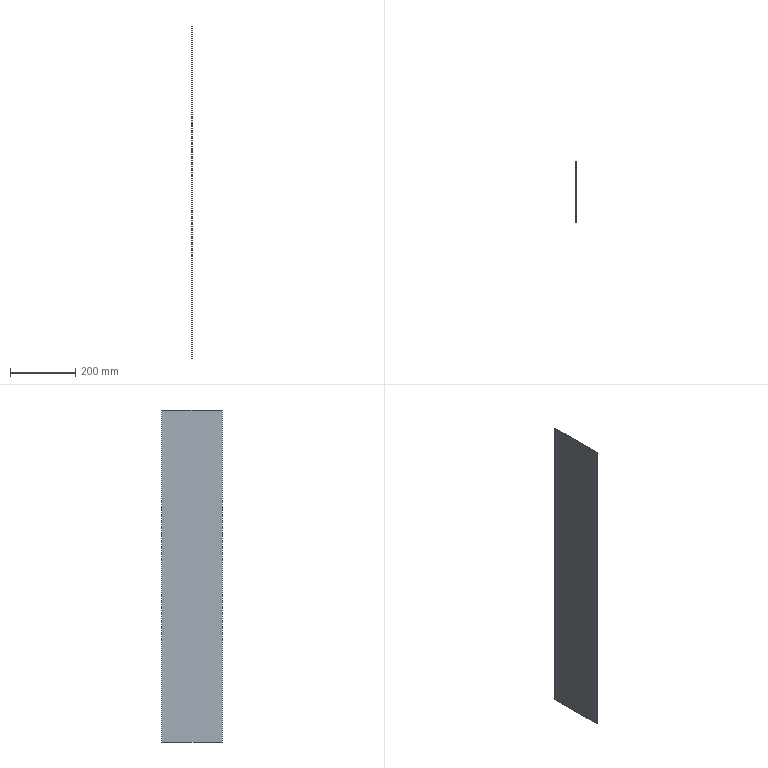Part | SolidWorks | 1 solid | 6 faces | box 1.5 x 185 x 1020 mm | volume 283050 mm3 | plane 6
STEP:
#1=CARTESIAN_POINT('',(0.,92.5,510.));
#2=VERTEX_POINT('',#1);
#3=CARTESIAN_POINT('',(0.,-92.5,510.));
#4=VERTEX_POINT('',#3);
#5=CARTESIAN_POINT('',(0.,-92.5,510.));
#6=DIRECTION('',(0.,-1.,0.));
#7=VECTOR('',#6,1000.);
#8=LINE('',#5,#7);
#9=EDGE_CURVE('',#2,#4,#8,.T.);
#10=ORIENTED_EDGE('',*,*,#9,.F.);
#11=CARTESIAN_POINT('',(-1.5,92.5,510.));
#12=VERTEX_POINT('',#11);
#13=CARTESIAN_POINT('',(-1.5,92.5,510.));
#14=DIRECTION('',(1.,0.,0.));
#15=VECTOR('',#14,1000.);
#16=LINE('',#13,#15);
#17=EDGE_CURVE('',#12,#2,#16,.T.);
#18=ORIENTED_EDGE('',*,*,#17,.F.);
#19=CARTESIAN_POINT('',(-1.5,-92.5,510.));
#20=VERTEX_POINT('',#19);
#21=CARTESIAN_POINT('',(-1.5,-92.5,510.));
#22=DIRECTION('',(0.,-1.,0.));
#23=VECTOR('',#22,1000.);
#24=LINE('',#21,#23);
#25=EDGE_CURVE('',#12,#20,#24,.T.);
#26=ORIENTED_EDGE('',*,*,#25,.T.);
#27=CARTESIAN_POINT('',(-1.5,-92.5,510.));
#28=DIRECTION('',(1.,0.,0.));
#29=VECTOR('',#28,1000.);
#30=LINE('',#27,#29);
#31=EDGE_CURVE('',#20,#4,#30,.T.);
#32=ORIENTED_EDGE('',*,*,#31,.T.);
#33=EDGE_LOOP('',(#10,#18,#26,#32));
#34=FACE_OUTER_BOUND('',#33,.T.);
#35=CARTESIAN_POINT('',(-1.5,-92.5,510.));
#36=DIRECTION('',(0.,0.,1.));
#37=DIRECTION('',(1.,0.,0.));
#38=AXIS2_PLACEMENT_3D('',#35,#36,#37);
#39=PLANE('',#38);
#40=ADVANCED_FACE('',(#34),#39,.T.);
#41=CARTESIAN_POINT('',(0.,92.5,-510.));
#42=VERTEX_POINT('',#41);
#43=CARTESIAN_POINT('',(0.,92.5,-510.));
#44=DIRECTION('',(0.,0.,1.));
#45=VECTOR('',#44,1000.);
#46=LINE('',#43,#45);
#47=EDGE_CURVE('',#42,#2,#46,.T.);
#48=ORIENTED_EDGE('',*,*,#47,.F.);
#49=CARTESIAN_POINT('',(-1.5,92.5,-510.));
#50=VERTEX_POINT('',#49);
#51=CARTESIAN_POINT('',(-1.5,92.5,-510.));
#52=DIRECTION('',(1.,0.,0.));
#53=VECTOR('',#52,1000.);
#54=LINE('',#51,#53);
#55=EDGE_CURVE('',#50,#42,#54,.T.);
#56=ORIENTED_EDGE('',*,*,#55,.F.);
#57=CARTESIAN_POINT('',(-1.5,92.5,-510.));
#58=DIRECTION('',(0.,0.,1.));
#59=VECTOR('',#58,1000.);
#60=LINE('',#57,#59);
#61=EDGE_CURVE('',#50,#12,#60,.T.);
#62=ORIENTED_EDGE('',*,*,#61,.T.);
#63=ORIENTED_EDGE('',*,*,#17,.T.);
#64=EDGE_LOOP('',(#48,#56,#62,#63));
#65=FACE_OUTER_BOUND('',#64,.T.);
#66=CARTESIAN_POINT('',(-1.5,92.5,-510.));
#67=DIRECTION('',(0.,1.,0.));
#68=DIRECTION('',(0.,0.,1.));
#69=AXIS2_PLACEMENT_3D('',#66,#67,#68);
#70=PLANE('',#69);
#71=ADVANCED_FACE('',(#65),#70,.T.);
#72=CARTESIAN_POINT('',(0.,-92.5,-510.));
#73=VERTEX_POINT('',#72);
#74=CARTESIAN_POINT('',(0.,-92.5,-510.));
#75=DIRECTION('',(0.,1.,0.));
#76=VECTOR('',#75,1000.);
#77=LINE('',#74,#76);
#78=EDGE_CURVE('',#73,#42,#77,.T.);
#79=ORIENTED_EDGE('',*,*,#78,.F.);
#80=CARTESIAN_POINT('',(-1.5,-92.5,-510.));
#81=VERTEX_POINT('',#80);
#82=CARTESIAN_POINT('',(-1.5,-92.5,-510.));
#83=DIRECTION('',(1.,0.,0.));
#84=VECTOR('',#83,1000.);
#85=LINE('',#82,#84);
#86=EDGE_CURVE('',#81,#73,#85,.T.);
#87=ORIENTED_EDGE('',*,*,#86,.F.);
#88=CARTESIAN_POINT('',(-1.5,-92.5,-510.));
#89=DIRECTION('',(0.,1.,0.));
#90=VECTOR('',#89,1000.);
#91=LINE('',#88,#90);
#92=EDGE_CURVE('',#81,#50,#91,.T.);
#93=ORIENTED_EDGE('',*,*,#92,.T.);
#94=ORIENTED_EDGE('',*,*,#55,.T.);
#95=EDGE_LOOP('',(#79,#87,#93,#94));
#96=FACE_OUTER_BOUND('',#95,.T.);
#97=CARTESIAN_POINT('',(-1.5,-92.5,-510.));
#98=DIRECTION('',(0.,0.,-1.));
#99=DIRECTION('',(-1.,0.,0.));
#100=AXIS2_PLACEMENT_3D('',#97,#98,#99);
#101=PLANE('',#100);
#102=ADVANCED_FACE('',(#96),#101,.T.);
#103=CARTESIAN_POINT('',(0.,-92.5,-510.));
#104=DIRECTION('',(0.,0.,-1.));
#105=VECTOR('',#104,1000.);
#106=LINE('',#103,#105);
#107=EDGE_CURVE('',#4,#73,#106,.T.);
#108=ORIENTED_EDGE('',*,*,#107,.F.);
#109=ORIENTED_EDGE('',*,*,#31,.F.);
#110=CARTESIAN_POINT('',(-1.5,-92.5,-510.));
#111=DIRECTION('',(0.,0.,-1.));
#112=VECTOR('',#111,1000.);
#113=LINE('',#110,#112);
#114=EDGE_CURVE('',#20,#81,#113,.T.);
#115=ORIENTED_EDGE('',*,*,#114,.T.);
#116=ORIENTED_EDGE('',*,*,#86,.T.);
#117=EDGE_LOOP('',(#108,#109,#115,#116));
#118=FACE_OUTER_BOUND('',#117,.T.);
#119=CARTESIAN_POINT('',(-1.5,-92.5,-510.));
#120=DIRECTION('',(0.,-1.,0.));
#121=DIRECTION('',(0.,0.,-1.));
#122=AXIS2_PLACEMENT_3D('',#119,#120,#121);
#123=PLANE('',#122);
#124=ADVANCED_FACE('',(#118),#123,.T.);
#125=ORIENTED_EDGE('',*,*,#25,.F.);
#126=ORIENTED_EDGE('',*,*,#61,.F.);
#127=ORIENTED_EDGE('',*,*,#92,.F.);
#128=ORIENTED_EDGE('',*,*,#114,.F.);
#129=EDGE_LOOP('',(#125,#126,#127,#128));
#130=FACE_OUTER_BOUND('',#129,.T.);
#131=CARTESIAN_POINT('',(-1.5,0.,0.));
#132=DIRECTION('',(1.,0.,0.));
#133=DIRECTION('',(0.,0.,-1.));
#134=AXIS2_PLACEMENT_3D('',#131,#132,#133);
#135=PLANE('',#134);
#136=ADVANCED_FACE('',(#130),#135,.F.);
#137=ORIENTED_EDGE('',*,*,#9,.T.);
#138=ORIENTED_EDGE('',*,*,#107,.T.);
#139=ORIENTED_EDGE('',*,*,#78,.T.);
#140=ORIENTED_EDGE('',*,*,#47,.T.);
#141=EDGE_LOOP('',(#137,#138,#139,#140));
#142=FACE_OUTER_BOUND('',#141,.T.);
#143=CARTESIAN_POINT('',(0.,0.,0.));
#144=DIRECTION('',(1.,0.,0.));
#145=DIRECTION('',(0.,0.,-1.));
#146=AXIS2_PLACEMENT_3D('',#143,#144,#145);
#147=PLANE('',#146);
#148=ADVANCED_FACE('',(#142),#147,.T.);
#149=CLOSED_SHELL('',(#40,#71,#102,#124,#136,#148));
#150=MANIFOLD_SOLID_BREP('',#149);
#151=CARTESIAN_POINT('',(0.,0.,0.));
#152=DIRECTION('',(0.,0.,1.));
#153=DIRECTION('',(1.,0.,0.));
#154=AXIS2_PLACEMENT_3D('',#151,#152,#153);
#155=(LENGTH_UNIT()NAMED_UNIT(*)SI_UNIT(.MILLI.,.METRE.));
#156=UNCERTAINTY_MEASURE_WITH_UNIT(LENGTH_MEASURE(0.00001),#155,'','');
#157=(NAMED_UNIT(*)PLANE_ANGLE_UNIT()SI_UNIT($,.RADIAN.));
#158=(NAMED_UNIT(*)SI_UNIT($,.STERADIAN.)SOLID_ANGLE_UNIT());
#159=(GEOMETRIC_REPRESENTATION_CONTEXT(3)GLOBAL_UNCERTAINTY_ASSIGNED_CONTEXT((#156))GLOBAL_UNIT_ASSIGNED_CONTEXT((#155,#157,#158))REPRESENTATION_CONTEXT('',''));
#160=ADVANCED_BREP_SHAPE_REPRESENTATION('',(#150,#154),#159);